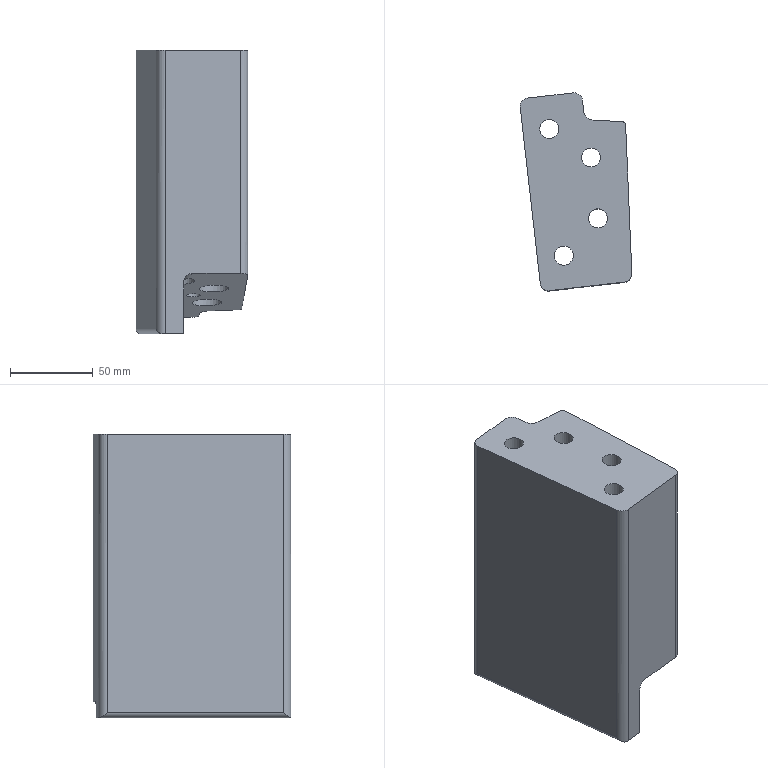Part | NX | features 8 2 | 1 solid | 36 faces | box 67.436 x 119.462 x 171 mm | volume 856634 mm3 | cylinder 19 | plane 15 | spline 1 | cone 1 | commonest cylinder face diameters 10 x7 11.5 x4 18 x4 4 x1 6 x1 8.5 x1
STEP:
#1=CARTESIAN_POINT('',(2963.913,339.568,91.));
#2=VERTEX_POINT('',#1);
#3=CARTESIAN_POINT('',(2958.163,339.568,91.));
#4=DIRECTION('',(0.,0.,-1.));
#5=DIRECTION('',(1.,0.,0.));
#6=AXIS2_PLACEMENT_3D('',#3,#4,#5);
#7=CIRCLE('',#6,5.75);
#8=EDGE_CURVE('',#2,#2,#7,.T.);
#9=ORIENTED_EDGE('',*,*,#8,.T.);
#10=EDGE_LOOP('',(#9));
#11=FACE_BOUND('',#10,.T.);
#12=CARTESIAN_POINT('',(2989.029,322.3,91.));
#13=VERTEX_POINT('',#12);
#14=CARTESIAN_POINT('',(2983.279,322.3,91.));
#15=DIRECTION('',(0.,0.,-1.));
#16=DIRECTION('',(1.,0.,0.));
#17=AXIS2_PLACEMENT_3D('',#14,#15,#16);
#18=CIRCLE('',#17,5.75);
#19=EDGE_CURVE('',#13,#13,#18,.T.);
#20=ORIENTED_EDGE('',*,*,#19,.T.);
#21=EDGE_LOOP('',(#20));
#22=FACE_BOUND('',#21,.T.);
#23=CARTESIAN_POINT('',(2958.215,241.946,91.));
#24=VERTEX_POINT('',#23);
#25=CARTESIAN_POINT('',(3003.536,247.11,91.));
#26=VERTEX_POINT('',#25);
#27=CARTESIAN_POINT('',(2988.519,245.399,91.));
#28=DIRECTION('',(0.9936,0.1132,0.));
#29=VECTOR('',#28,1000.);
#30=LINE('',#27,#29);
#31=EDGE_CURVE('',#24,#26,#30,.T.);
#32=ORIENTED_EDGE('',*,*,#31,.T.);
#33=CARTESIAN_POINT('',(3007.966,252.287,91.));
#34=VERTEX_POINT('',#33);
#35=CARTESIAN_POINT('',(3002.97,252.077,91.));
#36=DIRECTION('',(0.,0.,-1.));
#37=DIRECTION('',(1.,0.,0.));
#38=AXIS2_PLACEMENT_3D('',#35,#36,#37);
#39=CIRCLE('',#38,5.);
#40=EDGE_CURVE('',#34,#26,#39,.T.);
#41=ORIENTED_EDGE('',*,*,#40,.F.);
#42=CARTESIAN_POINT('',(3004.206,342.067,91.));
#43=VERTEX_POINT('',#42);
#44=CARTESIAN_POINT('',(3007.776,256.811,91.));
#45=DIRECTION('',(0.04184,-0.9991,0.));
#46=VECTOR('',#45,1000.);
#47=LINE('',#44,#46);
#48=EDGE_CURVE('',#43,#34,#47,.T.);
#49=ORIENTED_EDGE('',*,*,#48,.F.);
#50=CARTESIAN_POINT('',(3002.271,343.982,91.));
#51=VERTEX_POINT('',#50);
#52=CARTESIAN_POINT('',(3002.208,341.983,91.));
#53=DIRECTION('',(0.,0.,1.));
#54=DIRECTION('',(1.,0.,0.));
#55=AXIS2_PLACEMENT_3D('',#52,#53,#54);
#56=CIRCLE('',#55,2.);
#57=EDGE_CURVE('',#43,#51,#56,.T.);
#58=ORIENTED_EDGE('',*,*,#57,.T.);
#59=CARTESIAN_POINT('',(2984.567,344.856,91.));
#60=VERTEX_POINT('',#59);
#61=CARTESIAN_POINT('',(3002.271,343.982,91.));
#62=CARTESIAN_POINT('',(2996.365,344.168,91.));
#63=CARTESIAN_POINT('',(2990.468,344.547,91.));
#64=CARTESIAN_POINT('',(2984.567,344.856,91.));
#65=B_SPLINE_CURVE_WITH_KNOTS('',3,(#61,#62,#63,#64),.UNSPECIFIED.,.F.,.F.,(4,4),(0.,0.01772),.UNSPECIFIED.);
#66=EDGE_CURVE('',#51,#60,#65,.T.);
#67=ORIENTED_EDGE('',*,*,#66,.T.);
#68=CARTESIAN_POINT('',(2978.919,350.168,91.));
#69=VERTEX_POINT('',#68);
#70=CARTESIAN_POINT('',(2984.881,350.848,91.));
#71=DIRECTION('',(0.,0.,-1.));
#72=DIRECTION('',(1.,0.,0.));
#73=AXIS2_PLACEMENT_3D('',#70,#71,#72);
#74=CIRCLE('',#73,6.);
#75=EDGE_CURVE('',#60,#69,#74,.T.);
#76=ORIENTED_EDGE('',*,*,#75,.T.);
#77=CARTESIAN_POINT('',(2978.148,356.942,91.));
#78=VERTEX_POINT('',#77);
#79=CARTESIAN_POINT('',(3005.458,117.242,91.));
#80=DIRECTION('',(-0.1132,0.9936,0.));
#81=VECTOR('',#80,1000.);
#82=LINE('',#79,#81);
#83=EDGE_CURVE('',#69,#78,#82,.T.);
#84=ORIENTED_EDGE('',*,*,#83,.T.);
#85=CARTESIAN_POINT('',(2972.614,361.343,91.));
#86=VERTEX_POINT('',#85);
#87=CARTESIAN_POINT('',(2973.18,356.376,91.));
#88=DIRECTION('',(0.,0.,-1.));
#89=DIRECTION('',(1.,0.,0.));
#90=AXIS2_PLACEMENT_3D('',#87,#88,#89);
#91=CIRCLE('',#90,5.);
#92=EDGE_CURVE('',#86,#78,#91,.T.);
#93=ORIENTED_EDGE('',*,*,#92,.F.);
#94=CARTESIAN_POINT('',(2944.97,358.194,91.));
#95=VERTEX_POINT('',#94);
#96=CARTESIAN_POINT('',(2975.274,361.646,91.));
#97=DIRECTION('',(-0.9936,-0.1132,0.));
#98=VECTOR('',#97,1000.);
#99=LINE('',#96,#98);
#100=EDGE_CURVE('',#86,#95,#99,.T.);
#101=ORIENTED_EDGE('',*,*,#100,.T.);
#102=CARTESIAN_POINT('',(2940.568,352.66,91.));
#103=VERTEX_POINT('',#102);
#104=CARTESIAN_POINT('',(2945.536,353.226,91.));
#105=DIRECTION('',(0.,0.,-1.));
#106=DIRECTION('',(1.,0.,0.));
#107=AXIS2_PLACEMENT_3D('',#104,#105,#106);
#108=CIRCLE('',#107,5.);
#109=EDGE_CURVE('',#103,#95,#108,.T.);
#110=ORIENTED_EDGE('',*,*,#109,.F.);
#111=CARTESIAN_POINT('',(2952.681,246.348,91.));
#112=VERTEX_POINT('',#111);
#113=CARTESIAN_POINT('',(2946.568,300.001,91.));
#114=DIRECTION('',(0.1132,-0.9936,0.));
#115=VECTOR('',#114,1000.);
#116=LINE('',#113,#115);
#117=EDGE_CURVE('',#103,#112,#116,.T.);
#118=ORIENTED_EDGE('',*,*,#117,.T.);
#119=CARTESIAN_POINT('',(2957.649,246.914,91.));
#120=DIRECTION('',(0.,0.,-1.));
#121=DIRECTION('',(1.,0.,0.));
#122=AXIS2_PLACEMENT_3D('',#119,#120,#121);
#123=CIRCLE('',#122,5.);
#124=EDGE_CURVE('',#24,#112,#123,.T.);
#125=ORIENTED_EDGE('',*,*,#124,.F.);
#126=EDGE_LOOP('',(#32,#41,#49,#58,#67,#76,#84,#93,#101,#110,#118,#125));
#127=FACE_BOUND('',#126,.T.);
#128=CARTESIAN_POINT('',(2993.218,285.538,91.));
#129=VERTEX_POINT('',#128);
#130=CARTESIAN_POINT('',(2987.468,285.538,91.));
#131=DIRECTION('',(0.,0.,1.));
#132=DIRECTION('',(1.,0.,0.));
#133=AXIS2_PLACEMENT_3D('',#130,#131,#132);
#134=CIRCLE('',#133,5.75);
#135=EDGE_CURVE('',#129,#129,#134,.T.);
#136=ORIENTED_EDGE('',*,*,#135,.F.);
#137=EDGE_LOOP('',(#136));
#138=FACE_BOUND('',#137,.T.);
#139=CARTESIAN_POINT('',(2972.63,263.063,91.));
#140=VERTEX_POINT('',#139);
#141=CARTESIAN_POINT('',(2966.88,263.063,91.));
#142=DIRECTION('',(0.,0.,1.));
#143=DIRECTION('',(1.,0.,0.));
#144=AXIS2_PLACEMENT_3D('',#141,#142,#143);
#145=CIRCLE('',#144,5.75);
#146=EDGE_CURVE('',#140,#140,#145,.T.);
#147=ORIENTED_EDGE('',*,*,#146,.F.);
#148=EDGE_LOOP('',(#147));
#149=FACE_BOUND('',#148,.T.);
#150=CARTESIAN_POINT('',(282.5,-193.,91.));
#151=DIRECTION('',(0.,0.,1.));
#152=DIRECTION('',(-1.,0.,0.));
#153=AXIS2_PLACEMENT_3D('',#150,#151,#152);
#154=PLANE('',#153);
#155=ADVANCED_FACE('',(#11,#22,#127,#138,#149),#154,.T.);
#156=CARTESIAN_POINT('',(2972.695,256.193,-46.508));
#157=VERTEX_POINT('',#156);
#158=CARTESIAN_POINT('',(2974.112,243.757,-43.656));
#159=VERTEX_POINT('',#158);
#160=CARTESIAN_POINT('',(2960.178,366.055,-71.699));
#161=DIRECTION('',(0.1104,-0.9687,0.2221));
#162=VECTOR('',#161,1000.);
#163=LINE('',#160,#162);
#164=EDGE_CURVE('',#157,#159,#163,.T.);
#165=ORIENTED_EDGE('',*,*,#164,.T.);
#166=CARTESIAN_POINT('',(2969.144,243.191,-48.784));
#167=VERTEX_POINT('',#166);
#168=CARTESIAN_POINT('',(2974.112,243.757,-48.784));
#169=DIRECTION('',(0.1132,-0.9936,0.));
#170=DIRECTION('',(0.,0.,1.));
#171=AXIS2_PLACEMENT_3D('',#168,#169,#170);
#172=ELLIPSE('',#171,5.128,5.);
#173=EDGE_CURVE('',#159,#167,#172,.T.);
#174=ORIENTED_EDGE('',*,*,#173,.T.);
#175=CARTESIAN_POINT('',(2967.899,254.12,-51.29));
#176=VERTEX_POINT('',#175);
#177=CARTESIAN_POINT('',(2963.053,296.652,-61.043));
#178=DIRECTION('',(-0.1104,0.9687,-0.2221));
#179=VECTOR('',#178,1000.);
#180=LINE('',#177,#179);
#181=EDGE_CURVE('',#167,#176,#180,.T.);
#182=ORIENTED_EDGE('',*,*,#181,.T.);
#183=CARTESIAN_POINT('',(2972.695,256.193,-46.508));
#184=CARTESIAN_POINT('',(2972.177,255.755,-46.422));
#185=CARTESIAN_POINT('',(2971.019,254.986,-46.477));
#186=CARTESIAN_POINT('',(2969.305,254.351,-47.515));
#187=CARTESIAN_POINT('',(2968.162,254.145,-49.255));
#188=CARTESIAN_POINT('',(2967.899,254.12,-50.607));
#189=CARTESIAN_POINT('',(2967.899,254.12,-51.29));
#190=B_SPLINE_CURVE_WITH_KNOTS('',3,(#183,#184,#185,#186,#187,#188,#189),.UNSPECIFIED.,.F.,.F.,(4,1,1,1,4),(0.,0.002027,0.004054,0.006081,0.008107),.UNSPECIFIED.);
#191=EDGE_CURVE('',#157,#176,#190,.T.);
#192=ORIENTED_EDGE('',*,*,#191,.F.);
#193=EDGE_LOOP('',(#165,#174,#182,#192));
#194=FACE_BOUND('',#193,.T.);
#195=CARTESIAN_POINT('',(2960.303,364.952,-76.574));
#196=DIRECTION('',(0.1104,-0.9687,0.2221));
#197=DIRECTION('',(0.,-0.2235,-0.9747));
#198=AXIS2_PLACEMENT_3D('',#195,#196,#197);
#199=CYLINDRICAL_SURFACE('',#198,5.);
#200=ADVANCED_FACE('',(#194),#199,.F.);
#201=CARTESIAN_POINT('',(2943.03,357.553,-80.));
#202=VERTEX_POINT('',#201);
#203=CARTESIAN_POINT('',(2956.18,242.134,-80.));
#204=VERTEX_POINT('',#203);
#205=CARTESIAN_POINT('',(2949.549,300.34,-80.));
#206=DIRECTION('',(0.1132,-0.9936,0.));
#207=VECTOR('',#206,1000.);
#208=LINE('',#205,#207);
#209=EDGE_CURVE('',#202,#204,#208,.T.);
#210=ORIENTED_EDGE('',*,*,#209,.F.);
#211=CARTESIAN_POINT('',(2944.97,358.194,-80.));
#212=VERTEX_POINT('',#211);
#213=CARTESIAN_POINT('',(2945.536,353.226,-80.));
#214=DIRECTION('',(0.,0.,1.));
#215=DIRECTION('',(-1.,0.,0.));
#216=AXIS2_PLACEMENT_3D('',#213,#214,#215);
#217=CIRCLE('',#216,5.);
#218=EDGE_CURVE('',#212,#202,#217,.T.);
#219=ORIENTED_EDGE('',*,*,#218,.F.);
#220=CARTESIAN_POINT('',(2955.899,359.439,-80.));
#221=VERTEX_POINT('',#220);
#222=CARTESIAN_POINT('',(2975.274,361.646,-80.));
#223=DIRECTION('',(0.9936,0.1132,0.));
#224=VECTOR('',#223,1000.);
#225=LINE('',#222,#224);
#226=EDGE_CURVE('',#212,#221,#225,.T.);
#227=ORIENTED_EDGE('',*,*,#226,.T.);
#228=CARTESIAN_POINT('',(2957.144,348.51,-80.));
#229=VERTEX_POINT('',#228);
#230=CARTESIAN_POINT('',(2962.465,301.812,-80.));
#231=DIRECTION('',(-0.1132,0.9936,0.));
#232=VECTOR('',#231,1000.);
#233=LINE('',#230,#232);
#234=EDGE_CURVE('',#229,#221,#233,.T.);
#235=ORIENTED_EDGE('',*,*,#234,.F.);
#236=CARTESIAN_POINT('',(2959.182,330.625,-80.));
#237=VERTEX_POINT('',#236);
#238=CARTESIAN_POINT('',(2958.163,339.568,-80.));
#239=DIRECTION('',(0.,0.,1.));
#240=DIRECTION('',(0.9744,0.225,0.));
#241=AXIS2_PLACEMENT_3D('',#238,#239,#240);
#242=CIRCLE('',#241,9.);
#243=EDGE_CURVE('',#229,#237,#242,.T.);
#244=ORIENTED_EDGE('',*,*,#243,.T.);
#245=CARTESIAN_POINT('',(2965.861,272.005,-80.));
#246=VERTEX_POINT('',#245);
#247=CARTESIAN_POINT('',(2962.465,301.812,-80.));
#248=DIRECTION('',(-0.1132,0.9936,0.));
#249=VECTOR('',#248,1000.);
#250=LINE('',#247,#249);
#251=EDGE_CURVE('',#246,#237,#250,.T.);
#252=ORIENTED_EDGE('',*,*,#251,.F.);
#253=CARTESIAN_POINT('',(2967.899,254.12,-80.));
#254=VERTEX_POINT('',#253);
#255=CARTESIAN_POINT('',(2966.88,263.063,-80.));
#256=DIRECTION('',(0.,0.,-1.));
#257=DIRECTION('',(1.,0.,0.));
#258=AXIS2_PLACEMENT_3D('',#255,#256,#257);
#259=CIRCLE('',#258,9.);
#260=EDGE_CURVE('',#254,#246,#259,.T.);
#261=ORIENTED_EDGE('',*,*,#260,.F.);
#262=CARTESIAN_POINT('',(2969.144,243.191,-80.));
#263=VERTEX_POINT('',#262);
#264=CARTESIAN_POINT('',(2962.465,301.812,-80.));
#265=DIRECTION('',(-0.1132,0.9936,0.));
#266=VECTOR('',#265,1000.);
#267=LINE('',#264,#266);
#268=EDGE_CURVE('',#263,#254,#267,.T.);
#269=ORIENTED_EDGE('',*,*,#268,.F.);
#270=CARTESIAN_POINT('',(2958.215,241.946,-80.));
#271=VERTEX_POINT('',#270);
#272=CARTESIAN_POINT('',(2988.519,245.399,-80.));
#273=DIRECTION('',(-0.9936,-0.1132,0.));
#274=VECTOR('',#273,1000.);
#275=LINE('',#272,#274);
#276=EDGE_CURVE('',#263,#271,#275,.T.);
#277=ORIENTED_EDGE('',*,*,#276,.T.);
#278=CARTESIAN_POINT('',(2957.649,246.914,-80.));
#279=DIRECTION('',(0.,0.,1.));
#280=DIRECTION('',(-1.,0.,0.));
#281=AXIS2_PLACEMENT_3D('',#278,#279,#280);
#282=CIRCLE('',#281,5.);
#283=EDGE_CURVE('',#204,#271,#282,.T.);
#284=ORIENTED_EDGE('',*,*,#283,.F.);
#285=EDGE_LOOP('',(#210,#219,#227,#235,#244,#252,#261,#269,#277,#284));
#286=FACE_BOUND('',#285,.T.);
#287=CARTESIAN_POINT('',(2914.774,296.378,-80.));
#288=DIRECTION('',(0.,0.,-1.));
#289=DIRECTION('',(1.,0.,0.));
#290=AXIS2_PLACEMENT_3D('',#287,#288,#289);
#291=PLANE('',#290);
#292=ADVANCED_FACE('',(#286),#291,.T.);
#293=CARTESIAN_POINT('',(2975.596,297.82,-55.855));
#294=VERTEX_POINT('',#293);
#295=CARTESIAN_POINT('',(2975.115,302.042,-56.824));
#296=DIRECTION('',(0.02515,-0.2207,-0.975));
#297=DIRECTION('',(0.1104,-0.9687,0.2221));
#298=AXIS2_PLACEMENT_3D('',#295,#296,#297);
#299=ELLIPSE('',#298,4.359,4.25);
#300=EDGE_CURVE('',#294,#294,#299,.T.);
#301=ORIENTED_EDGE('',*,*,#300,.F.);
#302=EDGE_LOOP('',(#301));
#303=FACE_BOUND('',#302,.T.);
#304=CARTESIAN_POINT('',(2971.001,271.064,-49.917));
#305=VERTEX_POINT('',#304);
#306=CARTESIAN_POINT('',(2966.88,263.063,-48.213));
#307=DIRECTION('',(-0.02515,0.2207,0.975));
#308=DIRECTION('',(0.1104,-0.9687,0.2221));
#309=AXIS2_PLACEMENT_3D('',#306,#307,#308);
#310=ELLIPSE('',#309,9.231,9.);
#311=EDGE_CURVE('',#157,#305,#310,.T.);
#312=ORIENTED_EDGE('',*,*,#311,.T.);
#313=CARTESIAN_POINT('',(2965.743,317.211,-60.499));
#314=VERTEX_POINT('',#313);
#315=CARTESIAN_POINT('',(2960.178,366.055,-71.699));
#316=DIRECTION('',(0.1104,-0.9687,0.2221));
#317=VECTOR('',#316,1000.);
#318=LINE('',#315,#317);
#319=EDGE_CURVE('',#314,#305,#318,.T.);
#320=ORIENTED_EDGE('',*,*,#319,.F.);
#321=CARTESIAN_POINT('',(2965.727,317.352,-60.531));
#322=VERTEX_POINT('',#321);
#323=CARTESIAN_POINT('',(2965.735,317.281,-60.515));
#324=DIRECTION('',(0.1104,-0.9687,0.2221));
#325=VECTOR('',#324,1000.);
#326=LINE('',#323,#325);
#327=EDGE_CURVE('',#322,#314,#326,.T.);
#328=ORIENTED_EDGE('',*,*,#327,.F.);
#329=CARTESIAN_POINT('',(2963.978,332.698,-64.05));
#330=VERTEX_POINT('',#329);
#331=CARTESIAN_POINT('',(2960.178,366.055,-71.699));
#332=DIRECTION('',(0.1104,-0.9687,0.2221));
#333=VECTOR('',#332,1000.);
#334=LINE('',#331,#333);
#335=EDGE_CURVE('',#330,#322,#334,.T.);
#336=ORIENTED_EDGE('',*,*,#335,.F.);
#337=CARTESIAN_POINT('',(2962.284,347.569,-67.46));
#338=VERTEX_POINT('',#337);
#339=CARTESIAN_POINT('',(2958.163,339.568,-65.755));
#340=DIRECTION('',(-0.02515,0.2207,0.975));
#341=DIRECTION('',(0.1104,-0.9687,0.2221));
#342=AXIS2_PLACEMENT_3D('',#339,#340,#341);
#343=ELLIPSE('',#342,9.231,9.);
#344=EDGE_CURVE('',#330,#338,#343,.T.);
#345=ORIENTED_EDGE('',*,*,#344,.T.);
#346=CARTESIAN_POINT('',(2960.867,360.005,-70.311));
#347=VERTEX_POINT('',#346);
#348=CARTESIAN_POINT('',(2960.178,366.055,-71.699));
#349=DIRECTION('',(0.1104,-0.9687,0.2221));
#350=VECTOR('',#349,1000.);
#351=LINE('',#348,#350);
#352=EDGE_CURVE('',#347,#338,#351,.T.);
#353=ORIENTED_EDGE('',*,*,#352,.F.);
#354=CARTESIAN_POINT('',(2972.614,361.343,-70.311));
#355=VERTEX_POINT('',#354);
#356=CARTESIAN_POINT('',(2975.274,361.646,-70.311));
#357=DIRECTION('',(0.9936,0.1132,0.000000001));
#358=VECTOR('',#357,1000.);
#359=LINE('',#356,#358);
#360=EDGE_CURVE('',#347,#355,#359,.T.);
#361=ORIENTED_EDGE('',*,*,#360,.T.);
#362=CARTESIAN_POINT('',(2978.148,356.942,-69.172));
#363=VERTEX_POINT('',#362);
#364=CARTESIAN_POINT('',(2973.18,356.376,-69.172));
#365=DIRECTION('',(-0.02515,0.2207,0.975));
#366=DIRECTION('',(0.1104,-0.9687,0.2221));
#367=AXIS2_PLACEMENT_3D('',#364,#365,#366);
#368=ELLIPSE('',#367,5.128,5.);
#369=EDGE_CURVE('',#363,#355,#368,.T.);
#370=ORIENTED_EDGE('',*,*,#369,.F.);
#371=CARTESIAN_POINT('',(2978.919,350.168,-67.619));
#372=VERTEX_POINT('',#371);
#373=CARTESIAN_POINT('',(2976.892,367.96,-71.699));
#374=DIRECTION('',(0.1104,-0.9687,0.2221));
#375=VECTOR('',#374,1000.);
#376=LINE('',#373,#375);
#377=EDGE_CURVE('',#363,#372,#376,.T.);
#378=ORIENTED_EDGE('',*,*,#377,.T.);
#379=CARTESIAN_POINT('',(2984.567,344.856,-66.271));
#380=VERTEX_POINT('',#379);
#381=CARTESIAN_POINT('',(2984.881,350.848,-67.619));
#382=DIRECTION('',(-0.02515,0.2207,0.975));
#383=DIRECTION('',(0.1104,-0.9687,0.2221));
#384=AXIS2_PLACEMENT_3D('',#381,#382,#383);
#385=ELLIPSE('',#384,6.154,6.);
#386=EDGE_CURVE('',#372,#380,#385,.T.);
#387=ORIENTED_EDGE('',*,*,#386,.T.);
#388=CARTESIAN_POINT('',(3002.271,343.982,-65.617));
#389=VERTEX_POINT('',#388);
#390=CARTESIAN_POINT('',(3002.271,343.982,-65.617));
#391=CARTESIAN_POINT('',(2996.364,344.168,-65.811));
#392=CARTESIAN_POINT('',(2990.468,344.547,-66.049));
#393=CARTESIAN_POINT('',(2984.567,344.856,-66.271));
#394=B_SPLINE_CURVE_WITH_KNOTS('',3,(#390,#391,#392,#393),.UNSPECIFIED.,.F.,.F.,(4,4),(0.,0.01774),.UNSPECIFIED.);
#395=EDGE_CURVE('',#389,#380,#394,.T.);
#396=ORIENTED_EDGE('',*,*,#395,.F.);
#397=CARTESIAN_POINT('',(3004.206,342.067,-65.133));
#398=VERTEX_POINT('',#397);
#399=CARTESIAN_POINT('',(3002.208,341.983,-65.166));
#400=DIRECTION('',(0.02515,-0.2207,-0.975));
#401=DIRECTION('',(0.1104,-0.9687,0.2221));
#402=AXIS2_PLACEMENT_3D('',#399,#400,#401);
#403=ELLIPSE('',#402,2.051,2.);
#404=EDGE_CURVE('',#389,#398,#403,.T.);
#405=ORIENTED_EDGE('',*,*,#404,.T.);
#406=CARTESIAN_POINT('',(3007.966,252.287,-44.714));
#407=VERTEX_POINT('',#406);
#408=CARTESIAN_POINT('',(3004.684,330.662,-62.539));
#409=DIRECTION('',(-0.0408,0.9743,-0.2216));
#410=VECTOR('',#409,1000.);
#411=LINE('',#408,#410);
#412=EDGE_CURVE('',#407,#398,#411,.T.);
#413=ORIENTED_EDGE('',*,*,#412,.F.);
#414=CARTESIAN_POINT('',(3003.536,247.11,-43.656));
#415=VERTEX_POINT('',#414);
#416=CARTESIAN_POINT('',(3002.97,252.077,-44.795));
#417=DIRECTION('',(-0.02515,0.2207,0.975));
#418=DIRECTION('',(0.1104,-0.9687,0.2221));
#419=AXIS2_PLACEMENT_3D('',#416,#417,#418);
#420=ELLIPSE('',#419,5.128,5.);
#421=EDGE_CURVE('',#415,#407,#420,.T.);
#422=ORIENTED_EDGE('',*,*,#421,.F.);
#423=CARTESIAN_POINT('',(2988.519,245.399,-43.656));
#424=DIRECTION('',(-0.9936,-0.1132,-0.000000001));
#425=VECTOR('',#424,1000.);
#426=LINE('',#423,#425);
#427=EDGE_CURVE('',#415,#159,#426,.T.);
#428=ORIENTED_EDGE('',*,*,#427,.T.);
#429=ORIENTED_EDGE('',*,*,#164,.F.);
#430=EDGE_LOOP('',(#312,#320,#328,#336,#345,#353,#361,#370,#378,#387,#396,#405,#413,#422,#428,#429));
#431=FACE_BOUND('',#430,.T.);
#432=CARTESIAN_POINT('',(2984.298,313.358,-59.148));
#433=VERTEX_POINT('',#432);
#434=CARTESIAN_POINT('',(2983.279,322.3,-61.198));
#435=DIRECTION('',(-0.02515,0.2207,0.975));
#436=DIRECTION('',(0.1104,-0.9687,0.2221));
#437=AXIS2_PLACEMENT_3D('',#434,#435,#436);
#438=ELLIPSE('',#437,9.231,9.);
#439=EDGE_CURVE('',#433,#433,#438,.T.);
#440=ORIENTED_EDGE('',*,*,#439,.T.);
#441=EDGE_LOOP('',(#440));
#442=FACE_BOUND('',#441,.T.);
#443=CARTESIAN_POINT('',(2988.487,276.595,-50.719));
#444=VERTEX_POINT('',#443);
#445=CARTESIAN_POINT('',(2987.468,285.538,-52.769));
#446=DIRECTION('',(-0.02515,0.2207,0.975));
#447=DIRECTION('',(0.1104,-0.9687,0.2221));
#448=AXIS2_PLACEMENT_3D('',#445,#446,#447);
#449=ELLIPSE('',#448,9.231,9.);
#450=EDGE_CURVE('',#444,#444,#449,.T.);
#451=ORIENTED_EDGE('',*,*,#450,.T.);
#452=EDGE_LOOP('',(#451));
#453=FACE_BOUND('',#452,.T.);
#454=CARTESIAN_POINT('',(3013.211,372.098,-71.699));
#455=DIRECTION('',(0.02515,-0.2207,-0.975));
#456=DIRECTION('',(-0.1104,0.9687,-0.2221));
#457=AXIS2_PLACEMENT_3D('',#454,#455,#456);
#458=PLANE('',#457);
#459=ADVANCED_FACE('',(#303,#431,#442,#453),#458,.T.);
#460=CARTESIAN_POINT('',(2965.861,272.005,-55.391));
#461=VERTEX_POINT('',#460);
#462=CARTESIAN_POINT('',(2959.182,330.625,-68.833));
#463=VERTEX_POINT('',#462);
#464=CARTESIAN_POINT('',(2963.053,296.652,-61.043));
#465=DIRECTION('',(-0.1104,0.9687,-0.2221));
#466=VECTOR('',#465,1000.);
#467=LINE('',#464,#466);
#468=EDGE_CURVE('',#461,#463,#467,.T.);
#469=ORIENTED_EDGE('',*,*,#468,.T.);
#470=CARTESIAN_POINT('',(2963.978,332.698,-64.05));
#471=CARTESIAN_POINT('',(2963.461,332.26,-63.964));
#472=CARTESIAN_POINT('',(2962.302,331.491,-64.02));
#473=CARTESIAN_POINT('',(2960.589,330.856,-65.057));
#474=CARTESIAN_POINT('',(2959.446,330.65,-66.797));
#475=CARTESIAN_POINT('',(2959.182,330.625,-68.149));
#476=CARTESIAN_POINT('',(2959.182,330.625,-68.833));
#477=B_SPLINE_CURVE_WITH_KNOTS('',3,(#470,#471,#472,#473,#474,#475,#476),.UNSPECIFIED.,.F.,.F.,(4,1,1,1,4),(0.,0.002027,0.004054,0.006081,0.008107),.UNSPECIFIED.);
#478=EDGE_CURVE('',#330,#463,#477,.T.);
#479=ORIENTED_EDGE('',*,*,#478,.F.);
#480=ORIENTED_EDGE('',*,*,#335,.T.);
#481=ORIENTED_EDGE('',*,*,#327,.T.);
#482=ORIENTED_EDGE('',*,*,#319,.T.);
#483=CARTESIAN_POINT('',(2965.861,272.005,-55.391));
#484=CARTESIAN_POINT('',(2965.861,272.005,-53.985));
#485=CARTESIAN_POINT('',(2967.048,272.238,-51.231));
#486=CARTESIAN_POINT('',(2969.762,271.702,-50.094));
#487=CARTESIAN_POINT('',(2971.001,271.064,-49.917));
#488=B_SPLINE_CURVE_WITH_KNOTS('',3,(#483,#484,#485,#486,#487),.UNSPECIFIED.,.F.,.F.,(4,1,4),(0.,0.004158,0.008316),.UNSPECIFIED.);
#489=EDGE_CURVE('',#461,#305,#488,.T.);
#490=ORIENTED_EDGE('',*,*,#489,.F.);
#491=EDGE_LOOP('',(#469,#479,#480,#481,#482,#490));
#492=FACE_BOUND('',#491,.T.);
#493=CARTESIAN_POINT('',(2960.303,364.952,-76.574));
#494=DIRECTION('',(0.1104,-0.9687,0.2221));
#495=DIRECTION('',(0.,-0.2235,-0.9747));
#496=AXIS2_PLACEMENT_3D('',#493,#494,#495);
#497=CYLINDRICAL_SURFACE('',#496,5.);
#498=ADVANCED_FACE('',(#492),#497,.F.);
#499=ORIENTED_EDGE('',*,*,#251,.T.);
#500=CARTESIAN_POINT('',(2959.182,330.625,-80.));
#501=DIRECTION('',(0.,0.,-1.));
#502=VECTOR('',#501,1000.);
#503=LINE('',#500,#502);
#504=EDGE_CURVE('',#463,#237,#503,.T.);
#505=ORIENTED_EDGE('',*,*,#504,.F.);
#506=ORIENTED_EDGE('',*,*,#468,.F.);
#507=CARTESIAN_POINT('',(2965.861,272.005,-80.));
#508=DIRECTION('',(0.,0.,1.));
#509=VECTOR('',#508,1000.);
#510=LINE('',#507,#509);
#511=EDGE_CURVE('',#246,#461,#510,.T.);
#512=ORIENTED_EDGE('',*,*,#511,.F.);
#513=EDGE_LOOP('',(#499,#505,#506,#512));
#514=FACE_BOUND('',#513,.T.);
#515=CARTESIAN_POINT('',(2962.465,301.812,-37.747));
#516=DIRECTION('',(-0.9936,-0.1132,0.));
#517=DIRECTION('',(0.1132,-0.9936,0.));
#518=AXIS2_PLACEMENT_3D('',#515,#516,#517);
#519=PLANE('',#518);
#520=ADVANCED_FACE('',(#514),#519,.F.);
#521=ORIENTED_EDGE('',*,*,#181,.F.);
#522=CARTESIAN_POINT('',(2969.144,243.191,0.));
#523=DIRECTION('',(0.,0.,1.));
#524=VECTOR('',#523,1000.);
#525=LINE('',#522,#524);
#526=EDGE_CURVE('',#263,#167,#525,.T.);
#527=ORIENTED_EDGE('',*,*,#526,.F.);
#528=ORIENTED_EDGE('',*,*,#268,.T.);
#529=CARTESIAN_POINT('',(2967.899,254.12,-80.));
#530=DIRECTION('',(0.,0.,-1.));
#531=VECTOR('',#530,1000.);
#532=LINE('',#529,#531);
#533=EDGE_CURVE('',#176,#254,#532,.T.);
#534=ORIENTED_EDGE('',*,*,#533,.F.);
#535=EDGE_LOOP('',(#521,#527,#528,#534));
#536=FACE_BOUND('',#535,.T.);
#537=CARTESIAN_POINT('',(2962.465,301.812,-37.747));
#538=DIRECTION('',(-0.9936,-0.1132,0.));
#539=DIRECTION('',(0.1132,-0.9936,0.));
#540=AXIS2_PLACEMENT_3D('',#537,#538,#539);
#541=PLANE('',#540);
#542=ADVANCED_FACE('',(#536),#541,.F.);
#543=ORIENTED_EDGE('',*,*,#234,.T.);
#544=CARTESIAN_POINT('',(2955.899,359.439,-75.439));
#545=VERTEX_POINT('',#544);
#546=CARTESIAN_POINT('',(2955.899,359.439,0.));
#547=DIRECTION('',(0.,0.,1.));
#548=VECTOR('',#547,1000.);
#549=LINE('',#546,#548);
#550=EDGE_CURVE('',#221,#545,#549,.T.);
#551=ORIENTED_EDGE('',*,*,#550,.T.);
#552=CARTESIAN_POINT('',(2957.144,348.51,-72.933));
#553=VERTEX_POINT('',#552);
#554=CARTESIAN_POINT('',(2963.053,296.652,-61.043));
#555=DIRECTION('',(-0.1104,0.9687,-0.2221));
#556=VECTOR('',#555,1000.);
#557=LINE('',#554,#556);
#558=EDGE_CURVE('',#553,#545,#557,.T.);
#559=ORIENTED_EDGE('',*,*,#558,.F.);
#560=CARTESIAN_POINT('',(2957.144,348.51,-80.));
#561=DIRECTION('',(0.,0.,1.));
#562=VECTOR('',#561,1000.);
#563=LINE('',#560,#562);
#564=EDGE_CURVE('',#229,#553,#563,.T.);
#565=ORIENTED_EDGE('',*,*,#564,.F.);
#566=EDGE_LOOP('',(#543,#551,#559,#565));
#567=FACE_BOUND('',#566,.T.);
#568=CARTESIAN_POINT('',(2962.465,301.812,-37.747));
#569=DIRECTION('',(-0.9936,-0.1132,0.));
#570=DIRECTION('',(0.1132,-0.9936,0.));
#571=AXIS2_PLACEMENT_3D('',#568,#569,#570);
#572=PLANE('',#571);
#573=ADVANCED_FACE('',(#567),#572,.F.);
#574=ORIENTED_EDGE('',*,*,#40,.T.);
#575=CARTESIAN_POINT('',(3003.536,247.11,0.));
#576=DIRECTION('',(0.,0.,-1.));
#577=VECTOR('',#576,1000.);
#578=LINE('',#575,#577);
#579=EDGE_CURVE('',#26,#415,#578,.T.);
#580=ORIENTED_EDGE('',*,*,#579,.T.);
#581=ORIENTED_EDGE('',*,*,#421,.T.);
#582=CARTESIAN_POINT('',(3007.966,252.287,100.));
#583=DIRECTION('',(0.,0.,1.));
#584=VECTOR('',#583,1000.);
#585=LINE('',#582,#584);
#586=EDGE_CURVE('',#407,#34,#585,.T.);
#587=ORIENTED_EDGE('',*,*,#586,.T.);
#588=EDGE_LOOP('',(#574,#580,#581,#587));
#589=FACE_BOUND('',#588,.T.);
#590=CARTESIAN_POINT('',(3002.97,252.077,0.));
#591=DIRECTION('',(0.,0.,1.));
#592=DIRECTION('',(-1.,0.,0.));
#593=AXIS2_PLACEMENT_3D('',#590,#591,#592);
#594=CYLINDRICAL_SURFACE('',#593,5.);
#595=ADVANCED_FACE('',(#589),#594,.T.);
#596=ORIENTED_EDGE('',*,*,#412,.T.);
#597=CARTESIAN_POINT('',(3004.206,342.067,-401.711));
#598=DIRECTION('',(0.,0.,-1.));
#599=VECTOR('',#598,1000.);
#600=LINE('',#597,#599);
#601=EDGE_CURVE('',#43,#398,#600,.T.);
#602=ORIENTED_EDGE('',*,*,#601,.F.);
#603=ORIENTED_EDGE('',*,*,#48,.T.);
#604=ORIENTED_EDGE('',*,*,#586,.F.);
#605=EDGE_LOOP('',(#596,#602,#603,#604));
#606=FACE_BOUND('',#605,.T.);
#607=CARTESIAN_POINT('',(3007.776,256.811,-382.321));
#608=DIRECTION('',(-0.9991,-0.04184,0.));
#609=DIRECTION('',(0.04184,-0.9991,0.));
#610=AXIS2_PLACEMENT_3D('',#607,#608,#609);
#611=PLANE('',#610);
#612=ADVANCED_FACE('',(#606),#611,.F.);
#613=ORIENTED_EDGE('',*,*,#57,.F.);
#614=ORIENTED_EDGE('',*,*,#601,.T.);
#615=ORIENTED_EDGE('',*,*,#404,.F.);
#616=CARTESIAN_POINT('',(3002.271,343.982,-402.195));
#617=DIRECTION('',(0.,0.,-1.));
#618=VECTOR('',#617,1000.);
#619=LINE('',#616,#618);
#620=EDGE_CURVE('',#51,#389,#619,.T.);
#621=ORIENTED_EDGE('',*,*,#620,.F.);
#622=EDGE_LOOP('',(#613,#614,#615,#621));
#623=FACE_BOUND('',#622,.T.);
#624=CARTESIAN_POINT('',(3002.208,341.983,-401.744));
#625=DIRECTION('',(0.,0.,1.));
#626=DIRECTION('',(-1.,0.,0.));
#627=AXIS2_PLACEMENT_3D('',#624,#625,#626);
#628=CYLINDRICAL_SURFACE('',#627,2.);
#629=ADVANCED_FACE('',(#623),#628,.T.);
#630=ORIENTED_EDGE('',*,*,#66,.F.);
#631=ORIENTED_EDGE('',*,*,#620,.T.);
#632=ORIENTED_EDGE('',*,*,#395,.T.);
#633=CARTESIAN_POINT('',(2984.567,344.856,-402.849));
#634=DIRECTION('',(0.,0.,-1.));
#635=VECTOR('',#634,1000.);
#636=LINE('',#633,#635);
#637=EDGE_CURVE('',#60,#380,#636,.T.);
#638=ORIENTED_EDGE('',*,*,#637,.F.);
#639=EDGE_LOOP('',(#630,#631,#632,#638));
#640=FACE_BOUND('',#639,.T.);
#641=CARTESIAN_POINT('',(3002.271,343.982,-65.617));
#642=CARTESIAN_POINT('',(3002.271,343.982,92.598));
#643=CARTESIAN_POINT('',(2996.364,344.168,-65.811));
#644=CARTESIAN_POINT('',(2996.364,344.168,92.404));
#645=CARTESIAN_POINT('',(2990.468,344.547,-66.049));
#646=CARTESIAN_POINT('',(2990.468,344.547,92.166));
#647=CARTESIAN_POINT('',(2984.567,344.856,-66.271));
#648=CARTESIAN_POINT('',(2984.567,344.856,91.944));
#649=B_SPLINE_SURFACE_WITH_KNOTS('',3,1,((#641,#642),(#643,#644),(#645,#646),(#647,#648)),.SURF_OF_LINEAR_EXTRUSION.,.F.,.F.,.F.,(4,4),(2,2),(0.,1.),(0.,1.),.PIECEWISE_BEZIER_KNOTS.);
#650=ADVANCED_FACE('',(#640),#649,.T.);
#651=ORIENTED_EDGE('',*,*,#75,.F.);
#652=ORIENTED_EDGE('',*,*,#637,.T.);
#653=ORIENTED_EDGE('',*,*,#386,.F.);
#654=CARTESIAN_POINT('',(2978.919,350.168,-404.197));
#655=DIRECTION('',(0.,0.,-1.));
#656=VECTOR('',#655,1000.);
#657=LINE('',#654,#656);
#658=EDGE_CURVE('',#69,#372,#657,.T.);
#659=ORIENTED_EDGE('',*,*,#658,.F.);
#660=EDGE_LOOP('',(#651,#652,#653,#659));
#661=FACE_BOUND('',#660,.T.);
#662=CARTESIAN_POINT('',(2984.881,350.848,-404.197));
#663=DIRECTION('',(0.,0.,1.));
#664=DIRECTION('',(-1.,0.,0.));
#665=AXIS2_PLACEMENT_3D('',#662,#663,#664);
#666=CYLINDRICAL_SURFACE('',#665,6.);
#667=ADVANCED_FACE('',(#661),#666,.F.);
#668=ORIENTED_EDGE('',*,*,#83,.F.);
#669=ORIENTED_EDGE('',*,*,#658,.T.);
#670=ORIENTED_EDGE('',*,*,#377,.F.);
#671=CARTESIAN_POINT('',(2978.148,356.942,0.));
#672=DIRECTION('',(0.,0.,-1.));
#673=VECTOR('',#672,1000.);
#674=LINE('',#671,#673);
#675=EDGE_CURVE('',#78,#363,#674,.T.);
#676=ORIENTED_EDGE('',*,*,#675,.F.);
#677=EDGE_LOOP('',(#668,#669,#670,#676));
#678=FACE_BOUND('',#677,.T.);
#679=CARTESIAN_POINT('',(2978.919,350.168,-404.197));
#680=DIRECTION('',(-0.9936,-0.1132,0.));
#681=DIRECTION('',(0.1132,-0.9936,0.));
#682=AXIS2_PLACEMENT_3D('',#679,#680,#681);
#683=PLANE('',#682);
#684=ADVANCED_FACE('',(#678),#683,.F.);
#685=ORIENTED_EDGE('',*,*,#92,.T.);
#686=ORIENTED_EDGE('',*,*,#675,.T.);
#687=ORIENTED_EDGE('',*,*,#369,.T.);
#688=CARTESIAN_POINT('',(2972.614,361.343,100.));
#689=DIRECTION('',(0.,0.,1.));
#690=VECTOR('',#689,1000.);
#691=LINE('',#688,#690);
#692=EDGE_CURVE('',#355,#86,#691,.T.);
#693=ORIENTED_EDGE('',*,*,#692,.T.);
#694=EDGE_LOOP('',(#685,#686,#687,#693));
#695=FACE_BOUND('',#694,.T.);
#696=CARTESIAN_POINT('',(2973.18,356.376,-404.197));
#697=DIRECTION('',(0.,0.,1.));
#698=DIRECTION('',(-1.,0.,0.));
#699=AXIS2_PLACEMENT_3D('',#696,#697,#698);
#700=CYLINDRICAL_SURFACE('',#699,5.);
#701=ADVANCED_FACE('',(#695),#700,.T.);
#702=ORIENTED_EDGE('',*,*,#100,.F.);
#703=ORIENTED_EDGE('',*,*,#692,.F.);
#704=ORIENTED_EDGE('',*,*,#360,.F.);
#705=CARTESIAN_POINT('',(2960.867,360.005,-75.439));
#706=DIRECTION('',(-0.1132,0.9936,0.));
#707=DIRECTION('',(0.,0.,1.));
#708=AXIS2_PLACEMENT_3D('',#705,#706,#707);
#709=ELLIPSE('',#708,5.128,5.);
#710=EDGE_CURVE('',#545,#347,#709,.T.);
#711=ORIENTED_EDGE('',*,*,#710,.F.);
#712=ORIENTED_EDGE('',*,*,#550,.F.);
#713=ORIENTED_EDGE('',*,*,#226,.F.);
#714=CARTESIAN_POINT('',(2944.97,358.194,0.));
#715=DIRECTION('',(0.,0.,-1.));
#716=VECTOR('',#715,1000.);
#717=LINE('',#714,#716);
#718=EDGE_CURVE('',#95,#212,#717,.T.);
#719=ORIENTED_EDGE('',*,*,#718,.F.);
#720=EDGE_LOOP('',(#702,#703,#704,#711,#712,#713,#719));
#721=FACE_BOUND('',#720,.T.);
#722=CARTESIAN_POINT('',(2975.274,361.646,0.));
#723=DIRECTION('',(-0.1132,0.9936,0.));
#724=DIRECTION('',(0.,0.,1.));
#725=AXIS2_PLACEMENT_3D('',#722,#723,#724);
#726=PLANE('',#725);
#727=ADVANCED_FACE('',(#721),#726,.T.);
#728=ORIENTED_EDGE('',*,*,#276,.F.);
#729=ORIENTED_EDGE('',*,*,#526,.T.);
#730=ORIENTED_EDGE('',*,*,#173,.F.);
#731=ORIENTED_EDGE('',*,*,#427,.F.);
#732=ORIENTED_EDGE('',*,*,#579,.F.);
#733=ORIENTED_EDGE('',*,*,#31,.F.);
#734=CARTESIAN_POINT('',(2958.215,241.946,0.));
#735=DIRECTION('',(0.,0.,1.));
#736=VECTOR('',#735,1000.);
#737=LINE('',#734,#736);
#738=EDGE_CURVE('',#271,#24,#737,.T.);
#739=ORIENTED_EDGE('',*,*,#738,.F.);
#740=EDGE_LOOP('',(#728,#729,#730,#731,#732,#733,#739));
#741=FACE_BOUND('',#740,.T.);
#742=CARTESIAN_POINT('',(2988.519,245.399,0.));
#743=DIRECTION('',(0.1132,-0.9936,0.));
#744=DIRECTION('',(0.,0.,-1.));
#745=AXIS2_PLACEMENT_3D('',#742,#743,#744);
#746=PLANE('',#745);
#747=ADVANCED_FACE('',(#741),#746,.T.);
#748=ORIENTED_EDGE('',*,*,#117,.F.);
#749=CARTESIAN_POINT('',(2940.568,352.66,-77.));
#750=VERTEX_POINT('',#749);
#751=CARTESIAN_POINT('',(2940.568,352.66,0.));
#752=DIRECTION('',(0.,0.,1.));
#753=VECTOR('',#752,1000.);
#754=LINE('',#751,#753);
#755=EDGE_CURVE('',#750,#103,#754,.T.);
#756=ORIENTED_EDGE('',*,*,#755,.F.);
#757=CARTESIAN_POINT('',(2952.681,246.348,-77.));
#758=VERTEX_POINT('',#757);
#759=CARTESIAN_POINT('',(2946.568,300.001,-77.));
#760=DIRECTION('',(-0.1132,0.9936,0.));
#761=VECTOR('',#760,1000.);
#762=LINE('',#759,#761);
#763=EDGE_CURVE('',#758,#750,#762,.T.);
#764=ORIENTED_EDGE('',*,*,#763,.F.);
#765=CARTESIAN_POINT('',(2952.681,246.348,0.));
#766=DIRECTION('',(0.,0.,-1.));
#767=VECTOR('',#766,1000.);
#768=LINE('',#765,#767);
#769=EDGE_CURVE('',#112,#758,#768,.T.);
#770=ORIENTED_EDGE('',*,*,#769,.F.);
#771=EDGE_LOOP('',(#748,#756,#764,#770));
#772=FACE_BOUND('',#771,.T.);
#773=CARTESIAN_POINT('',(2946.568,300.001,0.));
#774=DIRECTION('',(-0.9936,-0.1132,0.));
#775=DIRECTION('',(0.,0.,-1.));
#776=AXIS2_PLACEMENT_3D('',#773,#774,#775);
#777=PLANE('',#776);
#778=ADVANCED_FACE('',(#772),#777,.T.);
#779=ORIENTED_EDGE('',*,*,#558,.T.);
#780=ORIENTED_EDGE('',*,*,#710,.T.);
#781=ORIENTED_EDGE('',*,*,#352,.T.);
#782=CARTESIAN_POINT('',(2957.144,348.51,-72.933));
#783=CARTESIAN_POINT('',(2957.144,348.51,-71.527));
#784=CARTESIAN_POINT('',(2958.331,348.743,-68.774));
#785=CARTESIAN_POINT('',(2961.045,348.207,-67.636));
#786=CARTESIAN_POINT('',(2962.284,347.569,-67.46));
#787=B_SPLINE_CURVE_WITH_KNOTS('',3,(#782,#783,#784,#785,#786),.UNSPECIFIED.,.F.,.F.,(4,1,4),(0.,0.004158,0.008316),.UNSPECIFIED.);
#788=EDGE_CURVE('',#553,#338,#787,.T.);
#789=ORIENTED_EDGE('',*,*,#788,.F.);
#790=EDGE_LOOP('',(#779,#780,#781,#789));
#791=FACE_BOUND('',#790,.T.);
#792=CARTESIAN_POINT('',(2960.303,364.952,-76.574));
#793=DIRECTION('',(0.1104,-0.9687,0.2221));
#794=DIRECTION('',(0.,-0.2235,-0.9747));
#795=AXIS2_PLACEMENT_3D('',#792,#793,#794);
#796=CYLINDRICAL_SURFACE('',#795,5.);
#797=ADVANCED_FACE('',(#791),#796,.F.);
#798=ORIENTED_EDGE('',*,*,#763,.T.);
#799=CARTESIAN_POINT('',(2943.03,357.553,-80.));
#800=CARTESIAN_POINT('',(2942.059,356.99,-80.));
#801=CARTESIAN_POINT('',(2940.696,355.314,-79.03));
#802=CARTESIAN_POINT('',(2940.469,353.527,-77.676));
#803=CARTESIAN_POINT('',(2940.568,352.66,-77.));
#804=B_SPLINE_CURVE_WITH_KNOTS('',3,(#799,#800,#801,#802,#803),.UNSPECIFIED.,.F.,.F.,(4,1,4),(0.,0.00331,0.006621),.UNSPECIFIED.);
#805=EDGE_CURVE('',#202,#750,#804,.T.);
#806=ORIENTED_EDGE('',*,*,#805,.F.);
#807=ORIENTED_EDGE('',*,*,#209,.T.);
#808=CARTESIAN_POINT('',(2956.18,242.134,-80.));
#809=CARTESIAN_POINT('',(2955.107,242.464,-80.));
#810=CARTESIAN_POINT('',(2953.403,243.79,-79.03));
#811=CARTESIAN_POINT('',(2952.78,245.481,-77.676));
#812=CARTESIAN_POINT('',(2952.681,246.348,-77.));
#813=B_SPLINE_CURVE_WITH_KNOTS('',3,(#808,#809,#810,#811,#812),.UNSPECIFIED.,.F.,.F.,(4,1,4),(0.,0.00331,0.006621),.UNSPECIFIED.);
#814=EDGE_CURVE('',#758,#204,#813,.F.);
#815=ORIENTED_EDGE('',*,*,#814,.F.);
#816=EDGE_LOOP('',(#798,#806,#807,#815));
#817=FACE_BOUND('',#816,.T.);
#818=CARTESIAN_POINT('',(2949.549,300.34,-77.));
#819=DIRECTION('',(-0.1132,0.9936,0.));
#820=DIRECTION('',(-0.9936,-0.1132,0.));
#821=AXIS2_PLACEMENT_3D('',#818,#819,#820);
#822=CYLINDRICAL_SURFACE('',#821,3.);
#823=ADVANCED_FACE('',(#817),#822,.T.);
#824=CARTESIAN_POINT('',(2989.029,322.3,61.));
#825=VERTEX_POINT('',#824);
#826=CARTESIAN_POINT('',(2983.279,322.3,61.));
#827=DIRECTION('',(0.,0.,1.));
#828=DIRECTION('',(1.,0.,0.));
#829=AXIS2_PLACEMENT_3D('',#826,#827,#828);
#830=CIRCLE('',#829,5.75);
#831=EDGE_CURVE('',#825,#825,#830,.T.);
#832=ORIENTED_EDGE('',*,*,#831,.F.);
#833=EDGE_LOOP('',(#832));
#834=FACE_BOUND('',#833,.T.);
#835=ORIENTED_EDGE('',*,*,#19,.F.);
#836=EDGE_LOOP('',(#835));
#837=FACE_BOUND('',#836,.T.);
#838=CARTESIAN_POINT('',(2983.279,322.3,-80.));
#839=DIRECTION('',(0.,0.,1.));
#840=DIRECTION('',(-0.9744,-0.225,0.));
#841=AXIS2_PLACEMENT_3D('',#838,#839,#840);
#842=CYLINDRICAL_SURFACE('',#841,5.75);
#843=ADVANCED_FACE('',(#834,#837),#842,.F.);
#844=ORIENTED_EDGE('',*,*,#831,.T.);
#845=EDGE_LOOP('',(#844));
#846=FACE_BOUND('',#845,.T.);
#847=CARTESIAN_POINT('',(2992.279,322.3,61.));
#848=VERTEX_POINT('',#847);
#849=CARTESIAN_POINT('',(2983.279,322.3,61.));
#850=DIRECTION('',(0.,0.,1.));
#851=DIRECTION('',(1.,0.,0.));
#852=AXIS2_PLACEMENT_3D('',#849,#850,#851);
#853=CIRCLE('',#852,9.);
#854=EDGE_CURVE('',#848,#848,#853,.T.);
#855=ORIENTED_EDGE('',*,*,#854,.F.);
#856=EDGE_LOOP('',(#855));
#857=FACE_BOUND('',#856,.T.);
#858=CARTESIAN_POINT('',(3002.428,326.494,61.));
#859=DIRECTION('',(0.,0.,1.));
#860=DIRECTION('',(-0.9936,-0.1132,0.));
#861=AXIS2_PLACEMENT_3D('',#858,#859,#860);
#862=PLANE('',#861);
#863=ADVANCED_FACE('',(#846,#857),#862,.F.);
#864=ORIENTED_EDGE('',*,*,#439,.F.);
#865=EDGE_LOOP('',(#864));
#866=FACE_BOUND('',#865,.T.);
#867=ORIENTED_EDGE('',*,*,#854,.T.);
#868=EDGE_LOOP('',(#867));
#869=FACE_BOUND('',#868,.T.);
#870=CARTESIAN_POINT('',(2983.279,322.3,-80.));
#871=DIRECTION('',(0.,0.,1.));
#872=DIRECTION('',(-0.9744,-0.225,0.));
#873=AXIS2_PLACEMENT_3D('',#870,#871,#872);
#874=CYLINDRICAL_SURFACE('',#873,9.);
#875=ADVANCED_FACE('',(#866,#869),#874,.F.);
#876=CARTESIAN_POINT('',(2967.163,339.568,61.));
#877=VERTEX_POINT('',#876);
#878=CARTESIAN_POINT('',(2958.163,339.568,61.));
#879=DIRECTION('',(0.,0.,1.));
#880=DIRECTION('',(1.,0.,0.));
#881=AXIS2_PLACEMENT_3D('',#878,#879,#880);
#882=CIRCLE('',#881,9.);
#883=EDGE_CURVE('',#877,#877,#882,.T.);
#884=ORIENTED_EDGE('',*,*,#883,.T.);
#885=EDGE_LOOP('',(#884));
#886=FACE_BOUND('',#885,.T.);
#887=ORIENTED_EDGE('',*,*,#478,.T.);
#888=ORIENTED_EDGE('',*,*,#504,.T.);
#889=ORIENTED_EDGE('',*,*,#243,.F.);
#890=ORIENTED_EDGE('',*,*,#564,.T.);
#891=ORIENTED_EDGE('',*,*,#788,.T.);
#892=ORIENTED_EDGE('',*,*,#344,.F.);
#893=EDGE_LOOP('',(#887,#888,#889,#890,#891,#892));
#894=FACE_BOUND('',#893,.T.);
#895=CARTESIAN_POINT('',(2958.163,339.568,-80.));
#896=DIRECTION('',(0.,0.,1.));
#897=DIRECTION('',(-0.9744,-0.225,0.));
#898=AXIS2_PLACEMENT_3D('',#895,#896,#897);
#899=CYLINDRICAL_SURFACE('',#898,9.);
#900=ADVANCED_FACE('',(#886,#894),#899,.F.);
#901=CARTESIAN_POINT('',(2963.913,339.568,61.));
#902=VERTEX_POINT('',#901);
#903=CARTESIAN_POINT('',(2958.163,339.568,61.));
#904=DIRECTION('',(0.,0.,1.));
#905=DIRECTION('',(1.,0.,0.));
#906=AXIS2_PLACEMENT_3D('',#903,#904,#905);
#907=CIRCLE('',#906,5.75);
#908=EDGE_CURVE('',#902,#902,#907,.T.);
#909=ORIENTED_EDGE('',*,*,#908,.F.);
#910=EDGE_LOOP('',(#909));
#911=FACE_BOUND('',#910,.T.);
#912=ORIENTED_EDGE('',*,*,#8,.F.);
#913=EDGE_LOOP('',(#912));
#914=FACE_BOUND('',#913,.T.);
#915=CARTESIAN_POINT('',(2958.163,339.568,-80.));
#916=DIRECTION('',(0.,0.,1.));
#917=DIRECTION('',(-0.9744,-0.225,0.));
#918=AXIS2_PLACEMENT_3D('',#915,#916,#917);
#919=CYLINDRICAL_SURFACE('',#918,5.75);
#920=ADVANCED_FACE('',(#911,#914),#919,.F.);
#921=ORIENTED_EDGE('',*,*,#908,.T.);
#922=EDGE_LOOP('',(#921));
#923=FACE_BOUND('',#922,.T.);
#924=ORIENTED_EDGE('',*,*,#883,.F.);
#925=EDGE_LOOP('',(#924));
#926=FACE_BOUND('',#925,.T.);
#927=CARTESIAN_POINT('',(3002.428,326.494,61.));
#928=DIRECTION('',(0.,0.,1.));
#929=DIRECTION('',(-0.9936,-0.1132,0.));
#930=AXIS2_PLACEMENT_3D('',#927,#928,#929);
#931=PLANE('',#930);
#932=ADVANCED_FACE('',(#923,#926),#931,.F.);
#933=CARTESIAN_POINT('',(2993.218,285.538,61.));
#934=VERTEX_POINT('',#933);
#935=CARTESIAN_POINT('',(2987.468,285.538,61.));
#936=DIRECTION('',(0.,0.,-1.));
#937=DIRECTION('',(1.,0.,0.));
#938=AXIS2_PLACEMENT_3D('',#935,#936,#937);
#939=CIRCLE('',#938,5.75);
#940=EDGE_CURVE('',#934,#934,#939,.T.);
#941=ORIENTED_EDGE('',*,*,#940,.T.);
#942=EDGE_LOOP('',(#941));
#943=FACE_BOUND('',#942,.T.);
#944=ORIENTED_EDGE('',*,*,#135,.T.);
#945=EDGE_LOOP('',(#944));
#946=FACE_BOUND('',#945,.T.);
#947=CARTESIAN_POINT('',(2987.468,285.538,-80.));
#948=DIRECTION('',(0.,0.,1.));
#949=DIRECTION('',(-1.,0.,0.));
#950=AXIS2_PLACEMENT_3D('',#947,#948,#949);
#951=CYLINDRICAL_SURFACE('',#950,5.75);
#952=ADVANCED_FACE('',(#943,#946),#951,.F.);
#953=ORIENTED_EDGE('',*,*,#940,.F.);
#954=EDGE_LOOP('',(#953));
#955=FACE_BOUND('',#954,.T.);
#956=CARTESIAN_POINT('',(2996.468,285.538,61.));
#957=VERTEX_POINT('',#956);
#958=CARTESIAN_POINT('',(2987.468,285.538,61.));
#959=DIRECTION('',(0.,0.,-1.));
#960=DIRECTION('',(1.,0.,0.));
#961=AXIS2_PLACEMENT_3D('',#958,#959,#960);
#962=CIRCLE('',#961,9.);
#963=EDGE_CURVE('',#957,#957,#962,.T.);
#964=ORIENTED_EDGE('',*,*,#963,.T.);
#965=EDGE_LOOP('',(#964));
#966=FACE_BOUND('',#965,.T.);
#967=CARTESIAN_POINT('',(3002.428,326.494,61.));
#968=DIRECTION('',(0.,0.,1.));
#969=DIRECTION('',(-0.9936,-0.1132,0.));
#970=AXIS2_PLACEMENT_3D('',#967,#968,#969);
#971=PLANE('',#970);
#972=ADVANCED_FACE('',(#955,#966),#971,.F.);
#973=ORIENTED_EDGE('',*,*,#450,.F.);
#974=EDGE_LOOP('',(#973));
#975=FACE_BOUND('',#974,.T.);
#976=ORIENTED_EDGE('',*,*,#963,.F.);
#977=EDGE_LOOP('',(#976));
#978=FACE_BOUND('',#977,.T.);
#979=CARTESIAN_POINT('',(2987.468,285.538,-80.));
#980=DIRECTION('',(0.,0.,1.));
#981=DIRECTION('',(-1.,0.,0.));
#982=AXIS2_PLACEMENT_3D('',#979,#980,#981);
#983=CYLINDRICAL_SURFACE('',#982,9.);
#984=ADVANCED_FACE('',(#975,#978),#983,.F.);
#985=CARTESIAN_POINT('',(2975.88,263.063,61.));
#986=VERTEX_POINT('',#985);
#987=CARTESIAN_POINT('',(2966.88,263.063,61.));
#988=DIRECTION('',(0.,0.,-1.));
#989=DIRECTION('',(1.,0.,0.));
#990=AXIS2_PLACEMENT_3D('',#987,#988,#989);
#991=CIRCLE('',#990,9.);
#992=EDGE_CURVE('',#986,#986,#991,.T.);
#993=ORIENTED_EDGE('',*,*,#992,.F.);
#994=EDGE_LOOP('',(#993));
#995=FACE_BOUND('',#994,.T.);
#996=ORIENTED_EDGE('',*,*,#260,.T.);
#997=ORIENTED_EDGE('',*,*,#511,.T.);
#998=ORIENTED_EDGE('',*,*,#489,.T.);
#999=ORIENTED_EDGE('',*,*,#311,.F.);
#1000=ORIENTED_EDGE('',*,*,#191,.T.);
#1001=ORIENTED_EDGE('',*,*,#533,.T.);
#1002=EDGE_LOOP('',(#996,#997,#998,#999,#1000,#1001));
#1003=FACE_BOUND('',#1002,.T.);
#1004=CARTESIAN_POINT('',(2966.88,263.063,-80.));
#1005=DIRECTION('',(0.,0.,1.));
#1006=DIRECTION('',(-1.,0.,0.));
#1007=AXIS2_PLACEMENT_3D('',#1004,#1005,#1006);
#1008=CYLINDRICAL_SURFACE('',#1007,9.);
#1009=ADVANCED_FACE('',(#995,#1003),#1008,.F.);
#1010=CARTESIAN_POINT('',(2972.63,263.063,61.));
#1011=VERTEX_POINT('',#1010);
#1012=CARTESIAN_POINT('',(2966.88,263.063,61.));
#1013=DIRECTION('',(0.,0.,-1.));
#1014=DIRECTION('',(1.,0.,0.));
#1015=AXIS2_PLACEMENT_3D('',#1012,#1013,#1014);
#1016=CIRCLE('',#1015,5.75);
#1017=EDGE_CURVE('',#1011,#1011,#1016,.T.);
#1018=ORIENTED_EDGE('',*,*,#1017,.T.);
#1019=EDGE_LOOP('',(#1018));
#1020=FACE_BOUND('',#1019,.T.);
#1021=ORIENTED_EDGE('',*,*,#146,.T.);
#1022=EDGE_LOOP('',(#1021));
#1023=FACE_BOUND('',#1022,.T.);
#1024=CARTESIAN_POINT('',(2966.88,263.063,-80.));
#1025=DIRECTION('',(0.,0.,1.));
#1026=DIRECTION('',(-1.,0.,0.));
#1027=AXIS2_PLACEMENT_3D('',#1024,#1025,#1026);
#1028=CYLINDRICAL_SURFACE('',#1027,5.75);
#1029=ADVANCED_FACE('',(#1020,#1023),#1028,.F.);
#1030=ORIENTED_EDGE('',*,*,#1017,.F.);
#1031=EDGE_LOOP('',(#1030));
#1032=FACE_BOUND('',#1031,.T.);
#1033=ORIENTED_EDGE('',*,*,#992,.T.);
#1034=EDGE_LOOP('',(#1033));
#1035=FACE_BOUND('',#1034,.T.);
#1036=CARTESIAN_POINT('',(3002.428,326.494,61.));
#1037=DIRECTION('',(0.,0.,1.));
#1038=DIRECTION('',(-0.9936,-0.1132,0.));
#1039=AXIS2_PLACEMENT_3D('',#1036,#1037,#1038);
#1040=PLANE('',#1039);
#1041=ADVANCED_FACE('',(#1032,#1035),#1040,.F.);
#1042=ORIENTED_EDGE('',*,*,#218,.T.);
#1043=ORIENTED_EDGE('',*,*,#805,.T.);
#1044=ORIENTED_EDGE('',*,*,#755,.T.);
#1045=ORIENTED_EDGE('',*,*,#109,.T.);
#1046=ORIENTED_EDGE('',*,*,#718,.T.);
#1047=EDGE_LOOP('',(#1042,#1043,#1044,#1045,#1046));
#1048=FACE_BOUND('',#1047,.T.);
#1049=CARTESIAN_POINT('',(2945.536,353.226,0.));
#1050=DIRECTION('',(0.,0.,1.));
#1051=DIRECTION('',(-1.,0.,0.));
#1052=AXIS2_PLACEMENT_3D('',#1049,#1050,#1051);
#1053=CYLINDRICAL_SURFACE('',#1052,5.);
#1054=ADVANCED_FACE('',(#1048),#1053,.T.);
#1055=ORIENTED_EDGE('',*,*,#814,.T.);
#1056=ORIENTED_EDGE('',*,*,#283,.T.);
#1057=ORIENTED_EDGE('',*,*,#738,.T.);
#1058=ORIENTED_EDGE('',*,*,#124,.T.);
#1059=ORIENTED_EDGE('',*,*,#769,.T.);
#1060=EDGE_LOOP('',(#1055,#1056,#1057,#1058,#1059));
#1061=FACE_BOUND('',#1060,.T.);
#1062=CARTESIAN_POINT('',(2957.649,246.914,0.));
#1063=DIRECTION('',(0.,0.,1.));
#1064=DIRECTION('',(-1.,0.,0.));
#1065=AXIS2_PLACEMENT_3D('',#1062,#1063,#1064);
#1066=CYLINDRICAL_SURFACE('',#1065,5.);
#1067=ADVANCED_FACE('',(#1061),#1066,.T.);
#1068=ORIENTED_EDGE('',*,*,#300,.T.);
#1069=EDGE_LOOP('',(#1068));
#1070=FACE_BOUND('',#1069,.T.);
#1071=CARTESIAN_POINT('',(2970.865,302.042,-30.074));
#1072=VERTEX_POINT('',#1071);
#1073=CARTESIAN_POINT('',(2975.115,302.042,-30.074));
#1074=DIRECTION('',(0.,0.,-1.));
#1075=DIRECTION('',(-1.,0.,0.));
#1076=AXIS2_PLACEMENT_3D('',#1073,#1074,#1075);
#1077=CIRCLE('',#1076,4.25);
#1078=EDGE_CURVE('',#1072,#1072,#1077,.T.);
#1079=ORIENTED_EDGE('',*,*,#1078,.F.);
#1080=EDGE_LOOP('',(#1079));
#1081=FACE_BOUND('',#1080,.T.);
#1082=CARTESIAN_POINT('',(2975.115,302.042,-59.824));
#1083=DIRECTION('',(0.,0.,1.));
#1084=DIRECTION('',(-1.,0.,0.));
#1085=AXIS2_PLACEMENT_3D('',#1082,#1083,#1084);
#1086=CYLINDRICAL_SURFACE('',#1085,4.25);
#1087=ADVANCED_FACE('',(#1070,#1081),#1086,.F.);
#1088=CARTESIAN_POINT('',(2975.115,302.042,-25.824));
#1089=VERTEX_POINT('',#1088);
#1090=VERTEX_LOOP('',#1089);
#1091=FACE_BOUND('',#1090,.T.);
#1092=ORIENTED_EDGE('',*,*,#1078,.T.);
#1093=EDGE_LOOP('',(#1092));
#1094=FACE_BOUND('',#1093,.T.);
#1095=CARTESIAN_POINT('',(2975.115,302.042,-30.073));
#1096=DIRECTION('',(0.,0.,-1.));
#1097=DIRECTION('',(1.,0.,0.));
#1098=AXIS2_PLACEMENT_3D('',#1095,#1096,#1097);
#1099=CONICAL_SURFACE('',#1098,4.25,0.7854);
#1100=ADVANCED_FACE('',(#1091,#1094),#1099,.F.);
#1101=CLOSED_SHELL('',(#155,#200,#292,#459,#498,#520,#542,#573,#595,#612,#629,#650,#667,#684,#701,#727,#747,#778,#797,#823,#843,#863,#875,#900,#920,#932,#952,#972,#984,#1009,#1029,#1041,#1054,#1067,#1087,#1100));
#1102=MANIFOLD_SOLID_BREP('',#1101);
#1103=(LENGTH_UNIT()NAMED_UNIT(*)SI_UNIT(.MILLI.,.METRE.));
#1104=UNCERTAINTY_MEASURE_WITH_UNIT(LENGTH_MEASURE(0.0508),#1103,'','');
#1105=(NAMED_UNIT(*)PLANE_ANGLE_UNIT()SI_UNIT($,.RADIAN.));
#1106=(NAMED_UNIT(*)SI_UNIT($,.STERADIAN.)SOLID_ANGLE_UNIT());
#1107=(GEOMETRIC_REPRESENTATION_CONTEXT(3)GLOBAL_UNCERTAINTY_ASSIGNED_CONTEXT((#1104))GLOBAL_UNIT_ASSIGNED_CONTEXT((#1103,#1105,#1106))REPRESENTATION_CONTEXT('',''));
#1108=ADVANCED_BREP_SHAPE_REPRESENTATION('',(#1102),#1107);